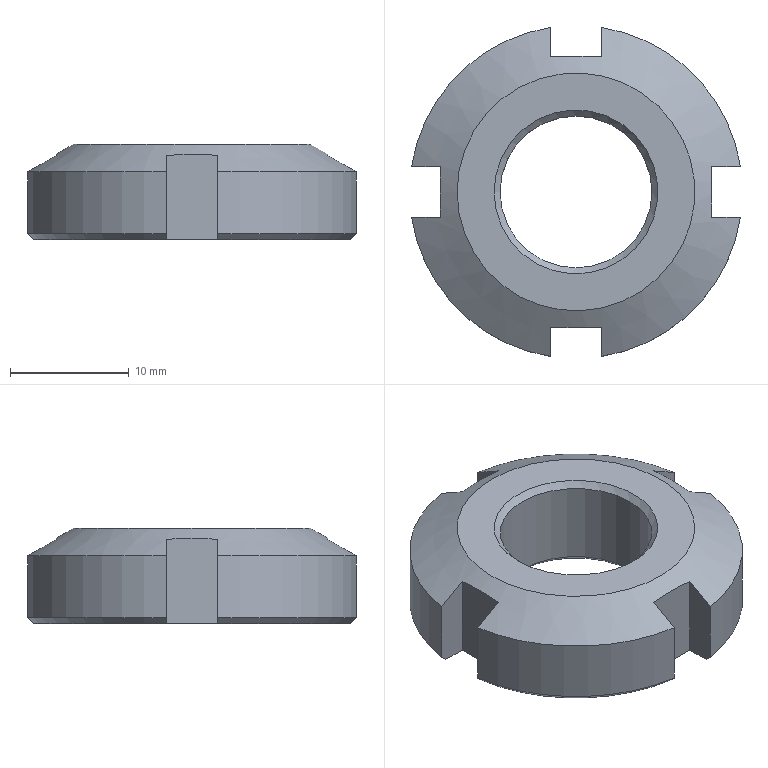Part | NX | features INSTANCE 4, CHAMFER 2, DATUM_CSYS 2, SKETCH 2, CIRCULAR_ISET 1, EXTRUDE 1, FSET 1, LINE 1, META 1, SWP104 1, SYMBOLIC_THREAD 1, THREADS 1, TRANSFORM_ISET 1 | 1 solid | 26 faces | box 27.668 x 27.668 x 8 mm | volume 3231 mm3 | plane 14 | cone 7 | cylinder 5 | commonest cylinder face diameters 28 x4 12.782 x1
STEP:
#1=CARTESIAN_POINT('',(-13.834,-2.15,0.5));
#2=VERTEX_POINT('',#1);
#3=CARTESIAN_POINT('',(-2.15,-13.834,0.5));
#4=VERTEX_POINT('',#3);
#5=CARTESIAN_POINT('',(0.,0.,0.5));
#6=DIRECTION('',(0.,0.,1.));
#7=DIRECTION('',(1.,0.,0.));
#8=AXIS2_PLACEMENT_3D('',#5,#6,#7);
#9=CIRCLE('',#8,14.);
#10=EDGE_CURVE('',#2,#4,#9,.T.);
#11=ORIENTED_EDGE('',*,*,#10,.T.);
#12=CARTESIAN_POINT('',(-2.15,-13.834,5.691));
#13=VERTEX_POINT('',#12);
#14=CARTESIAN_POINT('',(-2.15,-13.834,0.));
#15=DIRECTION('',(0.,0.,-1.));
#16=VECTOR('',#15,1000.);
#17=LINE('',#14,#16);
#18=EDGE_CURVE('',#4,#13,#17,.F.);
#19=ORIENTED_EDGE('',*,*,#18,.T.);
#20=CARTESIAN_POINT('',(-13.834,-2.15,5.691));
#21=VERTEX_POINT('',#20);
#22=CARTESIAN_POINT('',(0.,0.,5.691));
#23=DIRECTION('',(0.,0.,-1.));
#24=DIRECTION('',(-1.,0.,0.));
#25=AXIS2_PLACEMENT_3D('',#22,#23,#24);
#26=CIRCLE('',#25,14.);
#27=EDGE_CURVE('',#13,#21,#26,.T.);
#28=ORIENTED_EDGE('',*,*,#27,.T.);
#29=CARTESIAN_POINT('',(-13.834,-2.15,0.));
#30=DIRECTION('',(0.,0.,-1.));
#31=VECTOR('',#30,1000.);
#32=LINE('',#29,#31);
#33=EDGE_CURVE('',#21,#2,#32,.T.);
#34=ORIENTED_EDGE('',*,*,#33,.T.);
#35=EDGE_LOOP('',(#11,#19,#28,#34));
#36=FACE_BOUND('',#35,.T.);
#37=CARTESIAN_POINT('',(0.,0.,0.));
#38=DIRECTION('',(0.,0.,-1.));
#39=DIRECTION('',(-1.,0.,0.));
#40=AXIS2_PLACEMENT_3D('',#37,#38,#39);
#41=CYLINDRICAL_SURFACE('',#40,14.);
#42=ADVANCED_FACE('',(#36),#41,.T.);
#43=CARTESIAN_POINT('',(-2.15,-13.328,0.));
#44=VERTEX_POINT('',#43);
#45=CARTESIAN_POINT('',(-2.15,-13.834,0.5));
#46=CARTESIAN_POINT('',(-2.15,-13.665,0.3333));
#47=CARTESIAN_POINT('',(-2.15,-13.496,0.1666));
#48=CARTESIAN_POINT('',(-2.15,-13.328,0.));
#49=B_SPLINE_CURVE_WITH_KNOTS('',3,(#45,#46,#47,#48),.UNSPECIFIED.,.F.,.F.,(4,4),(0.004626,0.005337),.UNSPECIFIED.);
#50=EDGE_CURVE('',#4,#44,#49,.T.);
#51=ORIENTED_EDGE('',*,*,#50,.F.);
#52=ORIENTED_EDGE('',*,*,#10,.F.);
#53=CARTESIAN_POINT('',(-13.328,-2.15,0.));
#54=VERTEX_POINT('',#53);
#55=CARTESIAN_POINT('',(-13.328,-2.15,0.));
#56=CARTESIAN_POINT('',(-13.496,-2.15,0.1666));
#57=CARTESIAN_POINT('',(-13.665,-2.15,0.3333));
#58=CARTESIAN_POINT('',(-13.834,-2.15,0.5));
#59=B_SPLINE_CURVE_WITH_KNOTS('',3,(#55,#56,#57,#58),.UNSPECIFIED.,.F.,.F.,(4,4),(0.004492,0.005203),.UNSPECIFIED.);
#60=EDGE_CURVE('',#54,#2,#59,.T.);
#61=ORIENTED_EDGE('',*,*,#60,.F.);
#62=CARTESIAN_POINT('',(0.,0.,0.));
#63=DIRECTION('',(0.,0.,1.));
#64=DIRECTION('',(1.,0.,0.));
#65=AXIS2_PLACEMENT_3D('',#62,#63,#64);
#66=CIRCLE('',#65,13.5);
#67=EDGE_CURVE('',#44,#54,#66,.F.);
#68=ORIENTED_EDGE('',*,*,#67,.F.);
#69=EDGE_LOOP('',(#51,#52,#61,#68));
#70=FACE_BOUND('',#69,.T.);
#71=CARTESIAN_POINT('',(0.,0.,0.));
#72=DIRECTION('',(0.,0.,1.));
#73=DIRECTION('',(1.,0.,0.));
#74=AXIS2_PLACEMENT_3D('',#71,#72,#73);
#75=CONICAL_SURFACE('',#74,13.5,0.7854);
#76=ADVANCED_FACE('',(#70),#75,.T.);
#77=CARTESIAN_POINT('',(-2.15,13.834,0.5));
#78=VERTEX_POINT('',#77);
#79=CARTESIAN_POINT('',(-13.834,2.15,0.5));
#80=VERTEX_POINT('',#79);
#81=CARTESIAN_POINT('',(0.,0.,0.5));
#82=DIRECTION('',(0.,0.,1.));
#83=DIRECTION('',(1.,0.,0.));
#84=AXIS2_PLACEMENT_3D('',#81,#82,#83);
#85=CIRCLE('',#84,14.);
#86=EDGE_CURVE('',#78,#80,#85,.T.);
#87=ORIENTED_EDGE('',*,*,#86,.T.);
#88=CARTESIAN_POINT('',(-13.834,2.15,5.691));
#89=VERTEX_POINT('',#88);
#90=CARTESIAN_POINT('',(-13.834,2.15,0.));
#91=DIRECTION('',(0.,0.,-1.));
#92=VECTOR('',#91,1000.);
#93=LINE('',#90,#92);
#94=EDGE_CURVE('',#80,#89,#93,.F.);
#95=ORIENTED_EDGE('',*,*,#94,.T.);
#96=CARTESIAN_POINT('',(-2.15,13.834,5.691));
#97=VERTEX_POINT('',#96);
#98=CARTESIAN_POINT('',(0.,0.,5.691));
#99=DIRECTION('',(0.,0.,-1.));
#100=DIRECTION('',(-1.,0.,0.));
#101=AXIS2_PLACEMENT_3D('',#98,#99,#100);
#102=CIRCLE('',#101,14.);
#103=EDGE_CURVE('',#89,#97,#102,.T.);
#104=ORIENTED_EDGE('',*,*,#103,.T.);
#105=CARTESIAN_POINT('',(-2.15,13.834,0.));
#106=DIRECTION('',(0.,0.,-1.));
#107=VECTOR('',#106,1000.);
#108=LINE('',#105,#107);
#109=EDGE_CURVE('',#97,#78,#108,.T.);
#110=ORIENTED_EDGE('',*,*,#109,.T.);
#111=EDGE_LOOP('',(#87,#95,#104,#110));
#112=FACE_BOUND('',#111,.T.);
#113=CARTESIAN_POINT('',(0.,0.,0.));
#114=DIRECTION('',(0.,0.,-1.));
#115=DIRECTION('',(-1.,0.,0.));
#116=AXIS2_PLACEMENT_3D('',#113,#114,#115);
#117=CYLINDRICAL_SURFACE('',#116,14.);
#118=ADVANCED_FACE('',(#112),#117,.T.);
#119=CARTESIAN_POINT('',(-13.328,2.15,0.));
#120=VERTEX_POINT('',#119);
#121=CARTESIAN_POINT('',(-13.834,2.15,0.5));
#122=CARTESIAN_POINT('',(-13.665,2.15,0.3333));
#123=CARTESIAN_POINT('',(-13.496,2.15,0.1666));
#124=CARTESIAN_POINT('',(-13.328,2.15,0.));
#125=B_SPLINE_CURVE_WITH_KNOTS('',3,(#121,#122,#123,#124),.UNSPECIFIED.,.F.,.F.,(4,4),(0.004626,0.005337),.UNSPECIFIED.);
#126=EDGE_CURVE('',#80,#120,#125,.T.);
#127=ORIENTED_EDGE('',*,*,#126,.F.);
#128=ORIENTED_EDGE('',*,*,#86,.F.);
#129=CARTESIAN_POINT('',(-2.15,13.328,0.));
#130=VERTEX_POINT('',#129);
#131=CARTESIAN_POINT('',(-2.15,13.328,0.));
#132=CARTESIAN_POINT('',(-2.15,13.496,0.1666));
#133=CARTESIAN_POINT('',(-2.15,13.665,0.3333));
#134=CARTESIAN_POINT('',(-2.15,13.834,0.5));
#135=B_SPLINE_CURVE_WITH_KNOTS('',3,(#131,#132,#133,#134),.UNSPECIFIED.,.F.,.F.,(4,4),(0.004954,0.005666),.UNSPECIFIED.);
#136=EDGE_CURVE('',#130,#78,#135,.T.);
#137=ORIENTED_EDGE('',*,*,#136,.F.);
#138=CARTESIAN_POINT('',(0.,0.,0.));
#139=DIRECTION('',(0.,0.,1.));
#140=DIRECTION('',(1.,0.,0.));
#141=AXIS2_PLACEMENT_3D('',#138,#139,#140);
#142=CIRCLE('',#141,13.5);
#143=EDGE_CURVE('',#120,#130,#142,.F.);
#144=ORIENTED_EDGE('',*,*,#143,.F.);
#145=EDGE_LOOP('',(#127,#128,#137,#144));
#146=FACE_BOUND('',#145,.T.);
#147=CARTESIAN_POINT('',(0.,0.,0.));
#148=DIRECTION('',(0.,0.,1.));
#149=DIRECTION('',(1.,0.,0.));
#150=AXIS2_PLACEMENT_3D('',#147,#148,#149);
#151=CONICAL_SURFACE('',#150,13.5,0.7854);
#152=ADVANCED_FACE('',(#146),#151,.T.);
#153=CARTESIAN_POINT('',(13.834,2.15,0.5));
#154=VERTEX_POINT('',#153);
#155=CARTESIAN_POINT('',(2.15,13.834,0.5));
#156=VERTEX_POINT('',#155);
#157=CARTESIAN_POINT('',(0.,0.,0.5));
#158=DIRECTION('',(0.,0.,1.));
#159=DIRECTION('',(1.,0.,0.));
#160=AXIS2_PLACEMENT_3D('',#157,#158,#159);
#161=CIRCLE('',#160,14.);
#162=EDGE_CURVE('',#154,#156,#161,.T.);
#163=ORIENTED_EDGE('',*,*,#162,.T.);
#164=CARTESIAN_POINT('',(2.15,13.834,5.691));
#165=VERTEX_POINT('',#164);
#166=CARTESIAN_POINT('',(2.15,13.834,0.));
#167=DIRECTION('',(0.,0.,-1.));
#168=VECTOR('',#167,1000.);
#169=LINE('',#166,#168);
#170=EDGE_CURVE('',#156,#165,#169,.F.);
#171=ORIENTED_EDGE('',*,*,#170,.T.);
#172=CARTESIAN_POINT('',(13.834,2.15,5.691));
#173=VERTEX_POINT('',#172);
#174=CARTESIAN_POINT('',(0.,0.,5.691));
#175=DIRECTION('',(0.,0.,-1.));
#176=DIRECTION('',(-1.,0.,0.));
#177=AXIS2_PLACEMENT_3D('',#174,#175,#176);
#178=CIRCLE('',#177,14.);
#179=EDGE_CURVE('',#165,#173,#178,.T.);
#180=ORIENTED_EDGE('',*,*,#179,.T.);
#181=CARTESIAN_POINT('',(13.834,2.15,0.));
#182=DIRECTION('',(0.,0.,-1.));
#183=VECTOR('',#182,1000.);
#184=LINE('',#181,#183);
#185=EDGE_CURVE('',#173,#154,#184,.T.);
#186=ORIENTED_EDGE('',*,*,#185,.T.);
#187=EDGE_LOOP('',(#163,#171,#180,#186));
#188=FACE_BOUND('',#187,.T.);
#189=CARTESIAN_POINT('',(0.,0.,0.));
#190=DIRECTION('',(0.,0.,-1.));
#191=DIRECTION('',(-1.,0.,0.));
#192=AXIS2_PLACEMENT_3D('',#189,#190,#191);
#193=CYLINDRICAL_SURFACE('',#192,14.);
#194=ADVANCED_FACE('',(#188),#193,.T.);
#195=CARTESIAN_POINT('',(2.15,13.328,0.));
#196=VERTEX_POINT('',#195);
#197=CARTESIAN_POINT('',(2.15,13.834,0.5));
#198=CARTESIAN_POINT('',(2.15,13.665,0.3333));
#199=CARTESIAN_POINT('',(2.15,13.496,0.1666));
#200=CARTESIAN_POINT('',(2.15,13.328,0.));
#201=B_SPLINE_CURVE_WITH_KNOTS('',3,(#197,#198,#199,#200),.UNSPECIFIED.,.F.,.F.,(4,4),(0.004163,0.004875),.UNSPECIFIED.);
#202=EDGE_CURVE('',#156,#196,#201,.T.);
#203=ORIENTED_EDGE('',*,*,#202,.F.);
#204=ORIENTED_EDGE('',*,*,#162,.F.);
#205=CARTESIAN_POINT('',(13.328,2.15,0.));
#206=VERTEX_POINT('',#205);
#207=CARTESIAN_POINT('',(13.328,2.15,0.));
#208=CARTESIAN_POINT('',(13.496,2.15,0.1666));
#209=CARTESIAN_POINT('',(13.665,2.15,0.3333));
#210=CARTESIAN_POINT('',(13.834,2.15,0.5));
#211=B_SPLINE_CURVE_WITH_KNOTS('',3,(#207,#208,#209,#210),.UNSPECIFIED.,.F.,.F.,(4,4),(0.004954,0.005666),.UNSPECIFIED.);
#212=EDGE_CURVE('',#206,#154,#211,.T.);
#213=ORIENTED_EDGE('',*,*,#212,.F.);
#214=CARTESIAN_POINT('',(0.,0.,0.));
#215=DIRECTION('',(0.,0.,1.));
#216=DIRECTION('',(1.,0.,0.));
#217=AXIS2_PLACEMENT_3D('',#214,#215,#216);
#218=CIRCLE('',#217,13.5);
#219=EDGE_CURVE('',#196,#206,#218,.F.);
#220=ORIENTED_EDGE('',*,*,#219,.F.);
#221=EDGE_LOOP('',(#203,#204,#213,#220));
#222=FACE_BOUND('',#221,.T.);
#223=CARTESIAN_POINT('',(0.,0.,0.));
#224=DIRECTION('',(0.,0.,1.));
#225=DIRECTION('',(1.,0.,0.));
#226=AXIS2_PLACEMENT_3D('',#223,#224,#225);
#227=CONICAL_SURFACE('',#226,13.5,0.7854);
#228=ADVANCED_FACE('',(#222),#227,.T.);
#229=CARTESIAN_POINT('',(6.891,0.,0.));
#230=VERTEX_POINT('',#229);
#231=CARTESIAN_POINT('',(0.,0.,0.));
#232=DIRECTION('',(0.,0.,1.));
#233=DIRECTION('',(1.,0.,0.));
#234=AXIS2_PLACEMENT_3D('',#231,#232,#233);
#235=CIRCLE('',#234,6.891);
#236=EDGE_CURVE('',#230,#230,#235,.T.);
#237=ORIENTED_EDGE('',*,*,#236,.T.);
#238=EDGE_LOOP('',(#237));
#239=FACE_BOUND('',#238,.T.);
#240=CARTESIAN_POINT('',(-2.15,-11.4,0.));
#241=VERTEX_POINT('',#240);
#242=CARTESIAN_POINT('',(2.15,-11.4,0.));
#243=VERTEX_POINT('',#242);
#244=CARTESIAN_POINT('',(-2.15,-11.4,0.));
#245=DIRECTION('',(1.,0.,0.));
#246=VECTOR('',#245,1000.);
#247=LINE('',#244,#246);
#248=EDGE_CURVE('',#241,#243,#247,.T.);
#249=ORIENTED_EDGE('',*,*,#248,.F.);
#250=CARTESIAN_POINT('',(-2.15,-25.4,0.));
#251=DIRECTION('',(0.,1.,0.));
#252=VECTOR('',#251,1000.);
#253=LINE('',#250,#252);
#254=EDGE_CURVE('',#44,#241,#253,.T.);
#255=ORIENTED_EDGE('',*,*,#254,.F.);
#256=ORIENTED_EDGE('',*,*,#67,.T.);
#257=CARTESIAN_POINT('',(-11.4,-2.15,0.));
#258=VERTEX_POINT('',#257);
#259=CARTESIAN_POINT('',(-11.4,-2.15,0.));
#260=DIRECTION('',(-1.,0.,0.));
#261=VECTOR('',#260,1000.);
#262=LINE('',#259,#261);
#263=EDGE_CURVE('',#258,#54,#262,.T.);
#264=ORIENTED_EDGE('',*,*,#263,.F.);
#265=CARTESIAN_POINT('',(-11.4,2.15,0.));
#266=VERTEX_POINT('',#265);
#267=CARTESIAN_POINT('',(-11.4,2.15,0.));
#268=DIRECTION('',(0.,-1.,0.));
#269=VECTOR('',#268,1000.);
#270=LINE('',#267,#269);
#271=EDGE_CURVE('',#266,#258,#270,.T.);
#272=ORIENTED_EDGE('',*,*,#271,.F.);
#273=CARTESIAN_POINT('',(-25.4,2.15,0.));
#274=DIRECTION('',(1.,0.,0.));
#275=VECTOR('',#274,1000.);
#276=LINE('',#273,#275);
#277=EDGE_CURVE('',#120,#266,#276,.T.);
#278=ORIENTED_EDGE('',*,*,#277,.F.);
#279=ORIENTED_EDGE('',*,*,#143,.T.);
#280=CARTESIAN_POINT('',(-2.15,11.4,0.));
#281=VERTEX_POINT('',#280);
#282=CARTESIAN_POINT('',(-2.15,11.4,0.));
#283=DIRECTION('',(0.,1.,0.));
#284=VECTOR('',#283,1000.);
#285=LINE('',#282,#284);
#286=EDGE_CURVE('',#281,#130,#285,.T.);
#287=ORIENTED_EDGE('',*,*,#286,.F.);
#288=CARTESIAN_POINT('',(2.15,11.4,0.));
#289=VERTEX_POINT('',#288);
#290=CARTESIAN_POINT('',(2.15,11.4,0.));
#291=DIRECTION('',(-1.,0.,0.));
#292=VECTOR('',#291,1000.);
#293=LINE('',#290,#292);
#294=EDGE_CURVE('',#289,#281,#293,.T.);
#295=ORIENTED_EDGE('',*,*,#294,.F.);
#296=CARTESIAN_POINT('',(2.15,25.4,0.));
#297=DIRECTION('',(0.,-1.,0.));
#298=VECTOR('',#297,1000.);
#299=LINE('',#296,#298);
#300=EDGE_CURVE('',#196,#289,#299,.T.);
#301=ORIENTED_EDGE('',*,*,#300,.F.);
#302=ORIENTED_EDGE('',*,*,#219,.T.);
#303=CARTESIAN_POINT('',(11.4,2.15,0.));
#304=VERTEX_POINT('',#303);
#305=CARTESIAN_POINT('',(11.4,2.15,0.));
#306=DIRECTION('',(1.,0.,0.));
#307=VECTOR('',#306,1000.);
#308=LINE('',#305,#307);
#309=EDGE_CURVE('',#304,#206,#308,.T.);
#310=ORIENTED_EDGE('',*,*,#309,.F.);
#311=CARTESIAN_POINT('',(11.4,-2.15,0.));
#312=VERTEX_POINT('',#311);
#313=CARTESIAN_POINT('',(11.4,-2.15,0.));
#314=DIRECTION('',(0.,1.,0.));
#315=VECTOR('',#314,1000.);
#316=LINE('',#313,#315);
#317=EDGE_CURVE('',#312,#304,#316,.T.);
#318=ORIENTED_EDGE('',*,*,#317,.F.);
#319=CARTESIAN_POINT('',(13.328,-2.15,0.));
#320=VERTEX_POINT('',#319);
#321=CARTESIAN_POINT('',(25.4,-2.15,0.));
#322=DIRECTION('',(-1.,0.,0.));
#323=VECTOR('',#322,1000.);
#324=LINE('',#321,#323);
#325=EDGE_CURVE('',#320,#312,#324,.T.);
#326=ORIENTED_EDGE('',*,*,#325,.F.);
#327=CARTESIAN_POINT('',(2.15,-13.328,0.));
#328=VERTEX_POINT('',#327);
#329=CARTESIAN_POINT('',(0.,0.,0.));
#330=DIRECTION('',(0.,0.,1.));
#331=DIRECTION('',(1.,0.,0.));
#332=AXIS2_PLACEMENT_3D('',#329,#330,#331);
#333=CIRCLE('',#332,13.5);
#334=EDGE_CURVE('',#320,#328,#333,.F.);
#335=ORIENTED_EDGE('',*,*,#334,.T.);
#336=CARTESIAN_POINT('',(2.15,-11.4,0.));
#337=DIRECTION('',(0.,-1.,0.));
#338=VECTOR('',#337,1000.);
#339=LINE('',#336,#338);
#340=EDGE_CURVE('',#243,#328,#339,.T.);
#341=ORIENTED_EDGE('',*,*,#340,.F.);
#342=EDGE_LOOP('',(#249,#255,#256,#264,#272,#278,#279,#287,#295,#301,#302,#310,#318,#326,#335,#341));
#343=FACE_BOUND('',#342,.T.);
#344=CARTESIAN_POINT('',(14.,0.,0.));
#345=DIRECTION('',(0.,0.,1.));
#346=DIRECTION('',(1.,0.,0.));
#347=AXIS2_PLACEMENT_3D('',#344,#345,#346);
#348=PLANE('',#347);
#349=ADVANCED_FACE('',(#239,#343),#348,.F.);
#350=ORIENTED_EDGE('',*,*,#27,.F.);
#351=CARTESIAN_POINT('',(-2.15,-11.4,7.076));
#352=VERTEX_POINT('',#351);
#353=CARTESIAN_POINT('',(-2.15,-13.834,5.691));
#354=CARTESIAN_POINT('',(-2.15,-13.023,6.153));
#355=CARTESIAN_POINT('',(-2.15,-12.212,6.615));
#356=CARTESIAN_POINT('',(-2.15,-11.4,7.076));
#357=B_SPLINE_CURVE_WITH_KNOTS('',3,(#353,#354,#355,#356),.UNSPECIFIED.,.F.,.F.,(4,4),(0.006135,0.008936),.UNSPECIFIED.);
#358=EDGE_CURVE('',#13,#352,#357,.T.);
#359=ORIENTED_EDGE('',*,*,#358,.T.);
#360=CARTESIAN_POINT('',(2.15,-11.4,7.076));
#361=VERTEX_POINT('',#360);
#362=CARTESIAN_POINT('',(-2.15,-11.4,7.076));
#363=CARTESIAN_POINT('',(-0.7175,-11.4,7.229));
#364=CARTESIAN_POINT('',(0.7271,-11.4,7.228));
#365=CARTESIAN_POINT('',(2.15,-11.4,7.076));
#366=B_SPLINE_CURVE_WITH_KNOTS('',3,(#362,#363,#364,#365),.UNSPECIFIED.,.F.,.F.,(4,4),(0.009246,0.01352),.UNSPECIFIED.);
#367=EDGE_CURVE('',#352,#361,#366,.T.);
#368=ORIENTED_EDGE('',*,*,#367,.T.);
#369=CARTESIAN_POINT('',(2.15,-13.834,5.691));
#370=VERTEX_POINT('',#369);
#371=CARTESIAN_POINT('',(2.15,-11.4,7.076));
#372=CARTESIAN_POINT('',(2.15,-12.212,6.615));
#373=CARTESIAN_POINT('',(2.15,-13.023,6.153));
#374=CARTESIAN_POINT('',(2.15,-13.834,5.691));
#375=B_SPLINE_CURVE_WITH_KNOTS('',3,(#371,#372,#373,#374),.UNSPECIFIED.,.F.,.F.,(4,4),(0.003897,0.006697),.UNSPECIFIED.);
#376=EDGE_CURVE('',#361,#370,#375,.T.);
#377=ORIENTED_EDGE('',*,*,#376,.T.);
#378=CARTESIAN_POINT('',(13.834,-2.15,5.691));
#379=VERTEX_POINT('',#378);
#380=CARTESIAN_POINT('',(0.,0.,5.691));
#381=DIRECTION('',(0.,0.,-1.));
#382=DIRECTION('',(-1.,0.,0.));
#383=AXIS2_PLACEMENT_3D('',#380,#381,#382);
#384=CIRCLE('',#383,14.);
#385=EDGE_CURVE('',#379,#370,#384,.T.);
#386=ORIENTED_EDGE('',*,*,#385,.F.);
#387=CARTESIAN_POINT('',(11.4,-2.15,7.076));
#388=VERTEX_POINT('',#387);
#389=CARTESIAN_POINT('',(13.834,-2.15,5.691));
#390=CARTESIAN_POINT('',(13.023,-2.15,6.153));
#391=CARTESIAN_POINT('',(12.212,-2.15,6.615));
#392=CARTESIAN_POINT('',(11.4,-2.15,7.076));
#393=B_SPLINE_CURVE_WITH_KNOTS('',3,(#389,#390,#391,#392),.UNSPECIFIED.,.F.,.F.,(4,4),(0.004155,0.006955),.UNSPECIFIED.);
#394=EDGE_CURVE('',#379,#388,#393,.T.);
#395=ORIENTED_EDGE('',*,*,#394,.T.);
#396=CARTESIAN_POINT('',(11.4,2.15,7.076));
#397=VERTEX_POINT('',#396);
#398=CARTESIAN_POINT('',(11.4,-2.15,7.076));
#399=CARTESIAN_POINT('',(11.4,-0.7175,7.229));
#400=CARTESIAN_POINT('',(11.4,0.7271,7.228));
#401=CARTESIAN_POINT('',(11.4,2.15,7.076));
#402=B_SPLINE_CURVE_WITH_KNOTS('',3,(#398,#399,#400,#401),.UNSPECIFIED.,.F.,.F.,(4,4),(0.009246,0.01352),.UNSPECIFIED.);
#403=EDGE_CURVE('',#388,#397,#402,.T.);
#404=ORIENTED_EDGE('',*,*,#403,.T.);
#405=CARTESIAN_POINT('',(11.4,2.15,7.076));
#406=CARTESIAN_POINT('',(12.212,2.15,6.615));
#407=CARTESIAN_POINT('',(13.023,2.15,6.153));
#408=CARTESIAN_POINT('',(13.834,2.15,5.691));
#409=B_SPLINE_CURVE_WITH_KNOTS('',3,(#405,#406,#407,#408),.UNSPECIFIED.,.F.,.F.,(4,4),(0.005878,0.008678),.UNSPECIFIED.);
#410=EDGE_CURVE('',#397,#173,#409,.T.);
#411=ORIENTED_EDGE('',*,*,#410,.T.);
#412=ORIENTED_EDGE('',*,*,#179,.F.);
#413=CARTESIAN_POINT('',(2.15,11.4,7.076));
#414=VERTEX_POINT('',#413);
#415=CARTESIAN_POINT('',(2.15,13.834,5.691));
#416=CARTESIAN_POINT('',(2.15,13.023,6.153));
#417=CARTESIAN_POINT('',(2.15,12.212,6.615));
#418=CARTESIAN_POINT('',(2.15,11.4,7.076));
#419=B_SPLINE_CURVE_WITH_KNOTS('',3,(#415,#416,#417,#418),.UNSPECIFIED.,.F.,.F.,(4,4),(0.004155,0.006955),.UNSPECIFIED.);
#420=EDGE_CURVE('',#165,#414,#419,.T.);
#421=ORIENTED_EDGE('',*,*,#420,.T.);
#422=CARTESIAN_POINT('',(-2.15,11.4,7.076));
#423=VERTEX_POINT('',#422);
#424=CARTESIAN_POINT('',(2.15,11.4,7.076));
#425=CARTESIAN_POINT('',(0.7271,11.4,7.228));
#426=CARTESIAN_POINT('',(-0.7175,11.4,7.229));
#427=CARTESIAN_POINT('',(-2.15,11.4,7.076));
#428=B_SPLINE_CURVE_WITH_KNOTS('',3,(#424,#425,#426,#427),.UNSPECIFIED.,.F.,.F.,(4,4),(0.002509,0.0068),.UNSPECIFIED.);
#429=EDGE_CURVE('',#414,#423,#428,.T.);
#430=ORIENTED_EDGE('',*,*,#429,.T.);
#431=CARTESIAN_POINT('',(-2.15,11.4,7.076));
#432=CARTESIAN_POINT('',(-2.15,12.212,6.615));
#433=CARTESIAN_POINT('',(-2.15,13.023,6.153));
#434=CARTESIAN_POINT('',(-2.15,13.834,5.691));
#435=B_SPLINE_CURVE_WITH_KNOTS('',3,(#431,#432,#433,#434),.UNSPECIFIED.,.F.,.F.,(4,4),(0.005878,0.008678),.UNSPECIFIED.);
#436=EDGE_CURVE('',#423,#97,#435,.T.);
#437=ORIENTED_EDGE('',*,*,#436,.T.);
#438=ORIENTED_EDGE('',*,*,#103,.F.);
#439=CARTESIAN_POINT('',(-11.4,2.15,7.076));
#440=VERTEX_POINT('',#439);
#441=CARTESIAN_POINT('',(-13.834,2.15,5.691));
#442=CARTESIAN_POINT('',(-13.023,2.15,6.153));
#443=CARTESIAN_POINT('',(-12.212,2.15,6.615));
#444=CARTESIAN_POINT('',(-11.4,2.15,7.076));
#445=B_SPLINE_CURVE_WITH_KNOTS('',3,(#441,#442,#443,#444),.UNSPECIFIED.,.F.,.F.,(4,4),(0.006135,0.008936),.UNSPECIFIED.);
#446=EDGE_CURVE('',#89,#440,#445,.T.);
#447=ORIENTED_EDGE('',*,*,#446,.T.);
#448=CARTESIAN_POINT('',(-11.4,-2.15,7.076));
#449=VERTEX_POINT('',#448);
#450=CARTESIAN_POINT('',(-11.4,2.15,7.076));
#451=CARTESIAN_POINT('',(-11.4,0.7271,7.228));
#452=CARTESIAN_POINT('',(-11.4,-0.7175,7.229));
#453=CARTESIAN_POINT('',(-11.4,-2.15,7.076));
#454=B_SPLINE_CURVE_WITH_KNOTS('',3,(#450,#451,#452,#453),.UNSPECIFIED.,.F.,.F.,(4,4),(0.002509,0.0068),.UNSPECIFIED.);
#455=EDGE_CURVE('',#440,#449,#454,.T.);
#456=ORIENTED_EDGE('',*,*,#455,.T.);
#457=CARTESIAN_POINT('',(-11.4,-2.15,7.076));
#458=CARTESIAN_POINT('',(-12.212,-2.15,6.615));
#459=CARTESIAN_POINT('',(-13.023,-2.15,6.153));
#460=CARTESIAN_POINT('',(-13.834,-2.15,5.691));
#461=B_SPLINE_CURVE_WITH_KNOTS('',3,(#457,#458,#459,#460),.UNSPECIFIED.,.F.,.F.,(4,4),(0.003897,0.006697),.UNSPECIFIED.);
#462=EDGE_CURVE('',#449,#21,#461,.T.);
#463=ORIENTED_EDGE('',*,*,#462,.T.);
#464=EDGE_LOOP('',(#350,#359,#368,#377,#386,#395,#404,#411,#412,#421,#430,#437,#438,#447,#456,#463));
#465=FACE_BOUND('',#464,.T.);
#466=CARTESIAN_POINT('',(-10.,0.,8.));
#467=VERTEX_POINT('',#466);
#468=CARTESIAN_POINT('',(0.,0.,8.));
#469=DIRECTION('',(0.,0.,-1.));
#470=DIRECTION('',(-1.,0.,0.));
#471=AXIS2_PLACEMENT_3D('',#468,#469,#470);
#472=CIRCLE('',#471,10.);
#473=EDGE_CURVE('',#467,#467,#472,.T.);
#474=ORIENTED_EDGE('',*,*,#473,.T.);
#475=EDGE_LOOP('',(#474));
#476=FACE_BOUND('',#475,.T.);
#477=CARTESIAN_POINT('',(0.,0.,8.));
#478=DIRECTION('',(0.,0.,-1.));
#479=DIRECTION('',(-1.,0.,0.));
#480=AXIS2_PLACEMENT_3D('',#477,#478,#479);
#481=CONICAL_SURFACE('',#480,10.,1.047);
#482=ADVANCED_FACE('',(#465,#476),#481,.T.);
#483=ORIENTED_EDGE('',*,*,#385,.T.);
#484=CARTESIAN_POINT('',(2.15,-13.834,0.5));
#485=VERTEX_POINT('',#484);
#486=CARTESIAN_POINT('',(2.15,-13.834,0.));
#487=DIRECTION('',(0.,0.,-1.));
#488=VECTOR('',#487,1000.);
#489=LINE('',#486,#488);
#490=EDGE_CURVE('',#370,#485,#489,.T.);
#491=ORIENTED_EDGE('',*,*,#490,.T.);
#492=CARTESIAN_POINT('',(13.834,-2.15,0.5));
#493=VERTEX_POINT('',#492);
#494=CARTESIAN_POINT('',(0.,0.,0.5));
#495=DIRECTION('',(0.,0.,1.));
#496=DIRECTION('',(1.,0.,0.));
#497=AXIS2_PLACEMENT_3D('',#494,#495,#496);
#498=CIRCLE('',#497,14.);
#499=EDGE_CURVE('',#485,#493,#498,.T.);
#500=ORIENTED_EDGE('',*,*,#499,.T.);
#501=CARTESIAN_POINT('',(13.834,-2.15,0.));
#502=DIRECTION('',(0.,0.,-1.));
#503=VECTOR('',#502,1000.);
#504=LINE('',#501,#503);
#505=EDGE_CURVE('',#493,#379,#504,.F.);
#506=ORIENTED_EDGE('',*,*,#505,.T.);
#507=EDGE_LOOP('',(#483,#491,#500,#506));
#508=FACE_BOUND('',#507,.T.);
#509=CARTESIAN_POINT('',(0.,0.,0.));
#510=DIRECTION('',(0.,0.,-1.));
#511=DIRECTION('',(-1.,0.,0.));
#512=AXIS2_PLACEMENT_3D('',#509,#510,#511);
#513=CYLINDRICAL_SURFACE('',#512,14.);
#514=ADVANCED_FACE('',(#508),#513,.T.);
#515=CARTESIAN_POINT('',(6.391,0.,0.5));
#516=VERTEX_POINT('',#515);
#517=CARTESIAN_POINT('',(0.,0.,0.5));
#518=DIRECTION('',(0.,0.,1.));
#519=DIRECTION('',(1.,0.,0.));
#520=AXIS2_PLACEMENT_3D('',#517,#518,#519);
#521=CIRCLE('',#520,6.391);
#522=EDGE_CURVE('',#516,#516,#521,.F.);
#523=ORIENTED_EDGE('',*,*,#522,.T.);
#524=EDGE_LOOP('',(#523));
#525=FACE_BOUND('',#524,.T.);
#526=CARTESIAN_POINT('',(-6.391,0.,7.5));
#527=VERTEX_POINT('',#526);
#528=CARTESIAN_POINT('',(0.,0.,7.5));
#529=DIRECTION('',(0.,0.,-1.));
#530=DIRECTION('',(-1.,0.,0.));
#531=AXIS2_PLACEMENT_3D('',#528,#529,#530);
#532=CIRCLE('',#531,6.391);
#533=EDGE_CURVE('',#527,#527,#532,.F.);
#534=ORIENTED_EDGE('',*,*,#533,.T.);
#535=EDGE_LOOP('',(#534));
#536=FACE_BOUND('',#535,.T.);
#537=CARTESIAN_POINT('',(0.,0.,0.));
#538=DIRECTION('',(0.,0.,-1.));
#539=DIRECTION('',(-1.,0.,0.));
#540=AXIS2_PLACEMENT_3D('',#537,#538,#539);
#541=CYLINDRICAL_SURFACE('',#540,6.391);
#542=ADVANCED_FACE('',(#525,#536),#541,.F.);
#543=CARTESIAN_POINT('',(-6.891,0.,8.));
#544=VERTEX_POINT('',#543);
#545=CARTESIAN_POINT('',(0.,0.,8.));
#546=DIRECTION('',(0.,0.,-1.));
#547=DIRECTION('',(-1.,0.,0.));
#548=AXIS2_PLACEMENT_3D('',#545,#546,#547);
#549=CIRCLE('',#548,6.891);
#550=EDGE_CURVE('',#544,#544,#549,.T.);
#551=ORIENTED_EDGE('',*,*,#550,.T.);
#552=EDGE_LOOP('',(#551));
#553=FACE_BOUND('',#552,.T.);
#554=ORIENTED_EDGE('',*,*,#473,.F.);
#555=EDGE_LOOP('',(#554));
#556=FACE_BOUND('',#555,.T.);
#557=CARTESIAN_POINT('',(6.391,0.,8.));
#558=DIRECTION('',(0.,0.,-1.));
#559=DIRECTION('',(-1.,0.,0.));
#560=AXIS2_PLACEMENT_3D('',#557,#558,#559);
#561=PLANE('',#560);
#562=ADVANCED_FACE('',(#553,#556),#561,.F.);
#563=CARTESIAN_POINT('',(2.15,-13.328,0.));
#564=CARTESIAN_POINT('',(2.15,-13.496,0.1666));
#565=CARTESIAN_POINT('',(2.15,-13.665,0.3333));
#566=CARTESIAN_POINT('',(2.15,-13.834,0.5));
#567=B_SPLINE_CURVE_WITH_KNOTS('',3,(#563,#564,#565,#566),.UNSPECIFIED.,.F.,.F.,(4,4),(0.004492,0.005203),.UNSPECIFIED.);
#568=EDGE_CURVE('',#328,#485,#567,.T.);
#569=ORIENTED_EDGE('',*,*,#568,.F.);
#570=ORIENTED_EDGE('',*,*,#334,.F.);
#571=CARTESIAN_POINT('',(13.834,-2.15,0.5));
#572=CARTESIAN_POINT('',(13.665,-2.15,0.3333));
#573=CARTESIAN_POINT('',(13.496,-2.15,0.1666));
#574=CARTESIAN_POINT('',(13.328,-2.15,0.));
#575=B_SPLINE_CURVE_WITH_KNOTS('',3,(#571,#572,#573,#574),.UNSPECIFIED.,.F.,.F.,(4,4),(0.004163,0.004875),.UNSPECIFIED.);
#576=EDGE_CURVE('',#493,#320,#575,.T.);
#577=ORIENTED_EDGE('',*,*,#576,.F.);
#578=ORIENTED_EDGE('',*,*,#499,.F.);
#579=EDGE_LOOP('',(#569,#570,#577,#578));
#580=FACE_BOUND('',#579,.T.);
#581=CARTESIAN_POINT('',(0.,0.,0.));
#582=DIRECTION('',(0.,0.,1.));
#583=DIRECTION('',(1.,0.,0.));
#584=AXIS2_PLACEMENT_3D('',#581,#582,#583);
#585=CONICAL_SURFACE('',#584,13.5,0.7854);
#586=ADVANCED_FACE('',(#580),#585,.T.);
#587=ORIENTED_EDGE('',*,*,#236,.F.);
#588=EDGE_LOOP('',(#587));
#589=FACE_BOUND('',#588,.T.);
#590=ORIENTED_EDGE('',*,*,#522,.F.);
#591=EDGE_LOOP('',(#590));
#592=FACE_BOUND('',#591,.T.);
#593=CARTESIAN_POINT('',(0.,0.,0.5));
#594=DIRECTION('',(0.,0.,-1.));
#595=DIRECTION('',(-1.,0.,0.));
#596=AXIS2_PLACEMENT_3D('',#593,#594,#595);
#597=CONICAL_SURFACE('',#596,6.391,0.7854);
#598=ADVANCED_FACE('',(#589,#592),#597,.F.);
#599=ORIENTED_EDGE('',*,*,#533,.F.);
#600=EDGE_LOOP('',(#599));
#601=FACE_BOUND('',#600,.T.);
#602=ORIENTED_EDGE('',*,*,#550,.F.);
#603=EDGE_LOOP('',(#602));
#604=FACE_BOUND('',#603,.T.);
#605=CARTESIAN_POINT('',(0.,0.,8.));
#606=DIRECTION('',(0.,0.,1.));
#607=DIRECTION('',(1.,0.,0.));
#608=AXIS2_PLACEMENT_3D('',#605,#606,#607);
#609=CONICAL_SURFACE('',#608,6.891,0.7854);
#610=ADVANCED_FACE('',(#601,#604),#609,.F.);
#611=CARTESIAN_POINT('',(11.4,-2.15,8.));
#612=DIRECTION('',(0.,0.,-1.));
#613=VECTOR('',#612,1000.);
#614=LINE('',#611,#613);
#615=EDGE_CURVE('',#388,#312,#614,.T.);
#616=ORIENTED_EDGE('',*,*,#615,.T.);
#617=ORIENTED_EDGE('',*,*,#317,.T.);
#618=CARTESIAN_POINT('',(11.4,2.15,8.));
#619=DIRECTION('',(0.,0.,-1.));
#620=VECTOR('',#619,1000.);
#621=LINE('',#618,#620);
#622=EDGE_CURVE('',#397,#304,#621,.T.);
#623=ORIENTED_EDGE('',*,*,#622,.F.);
#624=ORIENTED_EDGE('',*,*,#403,.F.);
#625=EDGE_LOOP('',(#616,#617,#623,#624));
#626=FACE_BOUND('',#625,.T.);
#627=CARTESIAN_POINT('',(11.4,-2.15,8.));
#628=DIRECTION('',(-1.,0.,0.));
#629=DIRECTION('',(0.,0.,1.));
#630=AXIS2_PLACEMENT_3D('',#627,#628,#629);
#631=PLANE('',#630);
#632=ADVANCED_FACE('',(#626),#631,.F.);
#633=ORIENTED_EDGE('',*,*,#505,.F.);
#634=ORIENTED_EDGE('',*,*,#576,.T.);
#635=ORIENTED_EDGE('',*,*,#325,.T.);
#636=ORIENTED_EDGE('',*,*,#615,.F.);
#637=ORIENTED_EDGE('',*,*,#394,.F.);
#638=EDGE_LOOP('',(#633,#634,#635,#636,#637));
#639=FACE_BOUND('',#638,.T.);
#640=CARTESIAN_POINT('',(25.4,-2.15,8.));
#641=DIRECTION('',(0.,-1.,0.));
#642=DIRECTION('',(1.,0.,0.));
#643=AXIS2_PLACEMENT_3D('',#640,#641,#642);
#644=PLANE('',#643);
#645=ADVANCED_FACE('',(#639),#644,.F.);
#646=ORIENTED_EDGE('',*,*,#622,.T.);
#647=ORIENTED_EDGE('',*,*,#309,.T.);
#648=ORIENTED_EDGE('',*,*,#212,.T.);
#649=ORIENTED_EDGE('',*,*,#185,.F.);
#650=ORIENTED_EDGE('',*,*,#410,.F.);
#651=EDGE_LOOP('',(#646,#647,#648,#649,#650));
#652=FACE_BOUND('',#651,.T.);
#653=CARTESIAN_POINT('',(11.4,2.15,8.));
#654=DIRECTION('',(0.,1.,0.));
#655=DIRECTION('',(-1.,0.,0.));
#656=AXIS2_PLACEMENT_3D('',#653,#654,#655);
#657=PLANE('',#656);
#658=ADVANCED_FACE('',(#652),#657,.F.);
#659=CARTESIAN_POINT('',(2.15,11.4,8.));
#660=DIRECTION('',(0.,0.,-1.));
#661=VECTOR('',#660,1000.);
#662=LINE('',#659,#661);
#663=EDGE_CURVE('',#414,#289,#662,.T.);
#664=ORIENTED_EDGE('',*,*,#663,.T.);
#665=ORIENTED_EDGE('',*,*,#294,.T.);
#666=CARTESIAN_POINT('',(-2.15,11.4,8.));
#667=DIRECTION('',(0.,0.,-1.));
#668=VECTOR('',#667,1000.);
#669=LINE('',#666,#668);
#670=EDGE_CURVE('',#423,#281,#669,.T.);
#671=ORIENTED_EDGE('',*,*,#670,.F.);
#672=ORIENTED_EDGE('',*,*,#429,.F.);
#673=EDGE_LOOP('',(#664,#665,#671,#672));
#674=FACE_BOUND('',#673,.T.);
#675=CARTESIAN_POINT('',(2.15,11.4,8.));
#676=DIRECTION('',(0.,-1.,0.));
#677=DIRECTION('',(0.,0.,1.));
#678=AXIS2_PLACEMENT_3D('',#675,#676,#677);
#679=PLANE('',#678);
#680=ADVANCED_FACE('',(#674),#679,.F.);
#681=ORIENTED_EDGE('',*,*,#170,.F.);
#682=ORIENTED_EDGE('',*,*,#202,.T.);
#683=ORIENTED_EDGE('',*,*,#300,.T.);
#684=ORIENTED_EDGE('',*,*,#663,.F.);
#685=ORIENTED_EDGE('',*,*,#420,.F.);
#686=EDGE_LOOP('',(#681,#682,#683,#684,#685));
#687=FACE_BOUND('',#686,.T.);
#688=CARTESIAN_POINT('',(2.15,25.4,8.));
#689=DIRECTION('',(1.,0.,0.));
#690=DIRECTION('',(0.,1.,0.));
#691=AXIS2_PLACEMENT_3D('',#688,#689,#690);
#692=PLANE('',#691);
#693=ADVANCED_FACE('',(#687),#692,.F.);
#694=ORIENTED_EDGE('',*,*,#670,.T.);
#695=ORIENTED_EDGE('',*,*,#286,.T.);
#696=ORIENTED_EDGE('',*,*,#136,.T.);
#697=ORIENTED_EDGE('',*,*,#109,.F.);
#698=ORIENTED_EDGE('',*,*,#436,.F.);
#699=EDGE_LOOP('',(#694,#695,#696,#697,#698));
#700=FACE_BOUND('',#699,.T.);
#701=CARTESIAN_POINT('',(-2.15,11.4,8.));
#702=DIRECTION('',(-1.,0.,0.));
#703=DIRECTION('',(0.,-1.,0.));
#704=AXIS2_PLACEMENT_3D('',#701,#702,#703);
#705=PLANE('',#704);
#706=ADVANCED_FACE('',(#700),#705,.F.);
#707=CARTESIAN_POINT('',(-11.4,2.15,8.));
#708=DIRECTION('',(0.,0.,-1.));
#709=VECTOR('',#708,1000.);
#710=LINE('',#707,#709);
#711=EDGE_CURVE('',#440,#266,#710,.T.);
#712=ORIENTED_EDGE('',*,*,#711,.T.);
#713=ORIENTED_EDGE('',*,*,#271,.T.);
#714=CARTESIAN_POINT('',(-11.4,-2.15,8.));
#715=DIRECTION('',(0.,0.,-1.));
#716=VECTOR('',#715,1000.);
#717=LINE('',#714,#716);
#718=EDGE_CURVE('',#449,#258,#717,.T.);
#719=ORIENTED_EDGE('',*,*,#718,.F.);
#720=ORIENTED_EDGE('',*,*,#455,.F.);
#721=EDGE_LOOP('',(#712,#713,#719,#720));
#722=FACE_BOUND('',#721,.T.);
#723=CARTESIAN_POINT('',(-11.4,2.15,8.));
#724=DIRECTION('',(1.,0.,0.));
#725=DIRECTION('',(0.,0.,1.));
#726=AXIS2_PLACEMENT_3D('',#723,#724,#725);
#727=PLANE('',#726);
#728=ADVANCED_FACE('',(#722),#727,.F.);
#729=ORIENTED_EDGE('',*,*,#94,.F.);
#730=ORIENTED_EDGE('',*,*,#126,.T.);
#731=ORIENTED_EDGE('',*,*,#277,.T.);
#732=ORIENTED_EDGE('',*,*,#711,.F.);
#733=ORIENTED_EDGE('',*,*,#446,.F.);
#734=EDGE_LOOP('',(#729,#730,#731,#732,#733));
#735=FACE_BOUND('',#734,.T.);
#736=CARTESIAN_POINT('',(-25.4,2.15,8.));
#737=DIRECTION('',(0.,1.,0.));
#738=DIRECTION('',(-1.,0.,0.));
#739=AXIS2_PLACEMENT_3D('',#736,#737,#738);
#740=PLANE('',#739);
#741=ADVANCED_FACE('',(#735),#740,.F.);
#742=ORIENTED_EDGE('',*,*,#718,.T.);
#743=ORIENTED_EDGE('',*,*,#263,.T.);
#744=ORIENTED_EDGE('',*,*,#60,.T.);
#745=ORIENTED_EDGE('',*,*,#33,.F.);
#746=ORIENTED_EDGE('',*,*,#462,.F.);
#747=EDGE_LOOP('',(#742,#743,#744,#745,#746));
#748=FACE_BOUND('',#747,.T.);
#749=CARTESIAN_POINT('',(-11.4,-2.15,8.));
#750=DIRECTION('',(0.,-1.,0.));
#751=DIRECTION('',(1.,0.,0.));
#752=AXIS2_PLACEMENT_3D('',#749,#750,#751);
#753=PLANE('',#752);
#754=ADVANCED_FACE('',(#748),#753,.F.);
#755=CARTESIAN_POINT('',(-2.15,-11.4,8.));
#756=DIRECTION('',(0.,0.,-1.));
#757=VECTOR('',#756,1000.);
#758=LINE('',#755,#757);
#759=EDGE_CURVE('',#352,#241,#758,.T.);
#760=ORIENTED_EDGE('',*,*,#759,.T.);
#761=ORIENTED_EDGE('',*,*,#248,.T.);
#762=CARTESIAN_POINT('',(2.15,-11.4,8.));
#763=DIRECTION('',(0.,0.,-1.));
#764=VECTOR('',#763,1000.);
#765=LINE('',#762,#764);
#766=EDGE_CURVE('',#361,#243,#765,.T.);
#767=ORIENTED_EDGE('',*,*,#766,.F.);
#768=ORIENTED_EDGE('',*,*,#367,.F.);
#769=EDGE_LOOP('',(#760,#761,#767,#768));
#770=FACE_BOUND('',#769,.T.);
#771=CARTESIAN_POINT('',(-2.15,-11.4,8.));
#772=DIRECTION('',(0.,1.,0.));
#773=DIRECTION('',(0.,0.,1.));
#774=AXIS2_PLACEMENT_3D('',#771,#772,#773);
#775=PLANE('',#774);
#776=ADVANCED_FACE('',(#770),#775,.F.);
#777=ORIENTED_EDGE('',*,*,#18,.F.);
#778=ORIENTED_EDGE('',*,*,#50,.T.);
#779=ORIENTED_EDGE('',*,*,#254,.T.);
#780=ORIENTED_EDGE('',*,*,#759,.F.);
#781=ORIENTED_EDGE('',*,*,#358,.F.);
#782=EDGE_LOOP('',(#777,#778,#779,#780,#781));
#783=FACE_BOUND('',#782,.T.);
#784=CARTESIAN_POINT('',(-2.15,-25.4,8.));
#785=DIRECTION('',(-1.,0.,0.));
#786=DIRECTION('',(0.,-1.,0.));
#787=AXIS2_PLACEMENT_3D('',#784,#785,#786);
#788=PLANE('',#787);
#789=ADVANCED_FACE('',(#783),#788,.F.);
#790=ORIENTED_EDGE('',*,*,#766,.T.);
#791=ORIENTED_EDGE('',*,*,#340,.T.);
#792=ORIENTED_EDGE('',*,*,#568,.T.);
#793=ORIENTED_EDGE('',*,*,#490,.F.);
#794=ORIENTED_EDGE('',*,*,#376,.F.);
#795=EDGE_LOOP('',(#790,#791,#792,#793,#794));
#796=FACE_BOUND('',#795,.T.);
#797=CARTESIAN_POINT('',(2.15,-11.4,8.));
#798=DIRECTION('',(1.,0.,0.));
#799=DIRECTION('',(0.,1.,0.));
#800=AXIS2_PLACEMENT_3D('',#797,#798,#799);
#801=PLANE('',#800);
#802=ADVANCED_FACE('',(#796),#801,.F.);
#803=CLOSED_SHELL('',(#42,#76,#118,#152,#194,#228,#349,#482,#514,#542,#562,#586,#598,#610,#632,#645,#658,#680,#693,#706,#728,#741,#754,#776,#789,#802));
#804=MANIFOLD_SOLID_BREP('',#803);
#805=(LENGTH_UNIT()NAMED_UNIT(*)SI_UNIT(.MILLI.,.METRE.));
#806=UNCERTAINTY_MEASURE_WITH_UNIT(LENGTH_MEASURE(0.0508),#805,'','');
#807=(NAMED_UNIT(*)PLANE_ANGLE_UNIT()SI_UNIT($,.RADIAN.));
#808=(NAMED_UNIT(*)SI_UNIT($,.STERADIAN.)SOLID_ANGLE_UNIT());
#809=(GEOMETRIC_REPRESENTATION_CONTEXT(3)GLOBAL_UNCERTAINTY_ASSIGNED_CONTEXT((#806))GLOBAL_UNIT_ASSIGNED_CONTEXT((#805,#807,#808))REPRESENTATION_CONTEXT('',''));
#810=ADVANCED_BREP_SHAPE_REPRESENTATION('',(#804),#809);